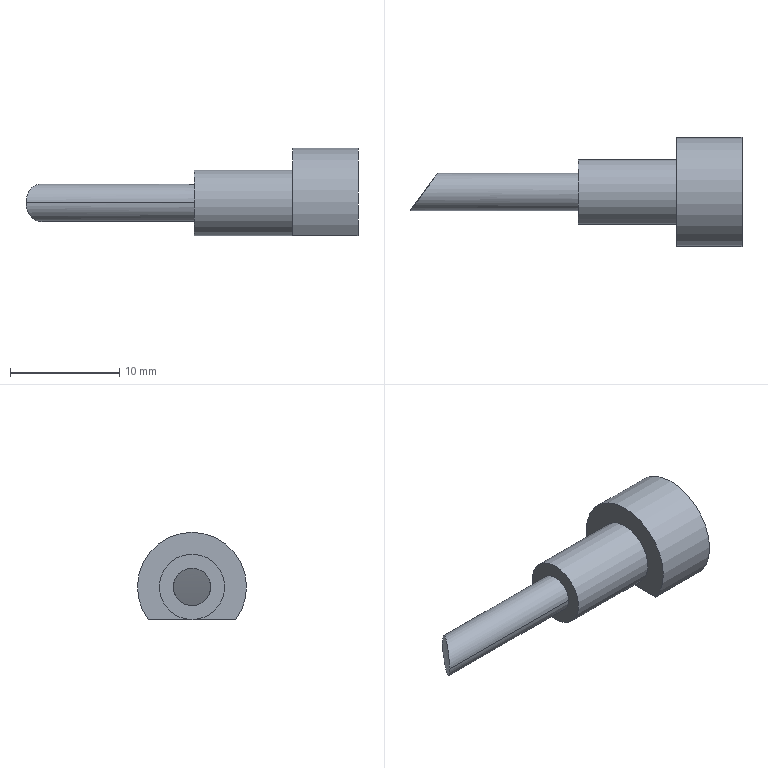Part | NX | features solid 2 | 1 solid | 9 faces | box 30.445 x 10 x 8 mm | volume 788.338 mm3 | cylinder 5 | plane 4 | commonest cylinder face diameters 3.417 x2 6 x1 10 x1 102.007 x1
STEP:
#1=CARTESIAN_POINT('',(64.275,-34.15,15.775));
#2=VERTEX_POINT('',#1);
#3=CARTESIAN_POINT('',(64.275,-26.15,15.775));
#4=VERTEX_POINT('',#3);
#5=CARTESIAN_POINT('',(64.275,-30.15,18.775));
#6=DIRECTION('',(-1.,0.,0.));
#7=DIRECTION('',(0.,0.,1.));
#8=AXIS2_PLACEMENT_3D('',#5,#6,#7);
#9=CIRCLE('',#8,5.);
#10=EDGE_CURVE('',#2,#4,#9,.T.);
#11=ORIENTED_EDGE('',*,*,#10,.F.);
#12=CARTESIAN_POINT('',(70.275,-34.15,15.775));
#13=VERTEX_POINT('',#12);
#14=CARTESIAN_POINT('',(70.275,-34.15,15.775));
#15=DIRECTION('',(-1.,0.,0.));
#16=VECTOR('',#15,1000.);
#17=LINE('',#14,#16);
#18=EDGE_CURVE('',#2,#13,#17,.F.);
#19=ORIENTED_EDGE('',*,*,#18,.T.);
#20=CARTESIAN_POINT('',(70.275,-26.15,15.775));
#21=VERTEX_POINT('',#20);
#22=CARTESIAN_POINT('',(70.275,-30.15,18.775));
#23=DIRECTION('',(-1.,0.,0.));
#24=DIRECTION('',(0.,0.,1.));
#25=AXIS2_PLACEMENT_3D('',#22,#23,#24);
#26=CIRCLE('',#25,5.);
#27=EDGE_CURVE('',#13,#21,#26,.T.);
#28=ORIENTED_EDGE('',*,*,#27,.T.);
#29=CARTESIAN_POINT('',(70.275,-26.15,15.775));
#30=DIRECTION('',(-1.,0.,0.));
#31=VECTOR('',#30,1000.);
#32=LINE('',#29,#31);
#33=EDGE_CURVE('',#21,#4,#32,.T.);
#34=ORIENTED_EDGE('',*,*,#33,.T.);
#35=EDGE_LOOP('',(#11,#19,#28,#34));
#36=FACE_BOUND('',#35,.T.);
#37=CARTESIAN_POINT('',(70.275,-30.15,18.775));
#38=DIRECTION('',(-1.,0.,0.));
#39=DIRECTION('',(0.,0.,1.));
#40=AXIS2_PLACEMENT_3D('',#37,#38,#39);
#41=CYLINDRICAL_SURFACE('',#40,5.);
#42=ADVANCED_FACE('',(#36),#41,.T.);
#43=CARTESIAN_POINT('',(64.275,-30.15,15.775));
#44=VERTEX_POINT('',#43);
#45=CARTESIAN_POINT('',(64.275,-30.15,18.775));
#46=DIRECTION('',(1.,0.,0.));
#47=DIRECTION('',(0.,0.,-1.));
#48=AXIS2_PLACEMENT_3D('',#45,#46,#47);
#49=CIRCLE('',#48,3.);
#50=EDGE_CURVE('',#44,#44,#49,.T.);
#51=ORIENTED_EDGE('',*,*,#50,.F.);
#52=EDGE_LOOP('',(#51));
#53=FACE_BOUND('',#52,.T.);
#54=CARTESIAN_POINT('',(55.275,-30.15,15.775));
#55=VERTEX_POINT('',#54);
#56=CARTESIAN_POINT('',(55.275,-30.15,18.775));
#57=DIRECTION('',(1.,0.,0.));
#58=DIRECTION('',(0.,0.,-1.));
#59=AXIS2_PLACEMENT_3D('',#56,#57,#58);
#60=CIRCLE('',#59,3.);
#61=EDGE_CURVE('',#55,#55,#60,.F.);
#62=ORIENTED_EDGE('',*,*,#61,.F.);
#63=EDGE_LOOP('',(#62));
#64=FACE_BOUND('',#63,.T.);
#65=CARTESIAN_POINT('',(-39.725,-30.15,18.775));
#66=DIRECTION('',(1.,0.,0.));
#67=DIRECTION('',(0.,0.,-1.));
#68=AXIS2_PLACEMENT_3D('',#65,#66,#67);
#69=CYLINDRICAL_SURFACE('',#68,3.);
#70=ADVANCED_FACE('',(#53,#64),#69,.T.);
#71=ORIENTED_EDGE('',*,*,#61,.T.);
#72=EDGE_LOOP('',(#71));
#73=FACE_BOUND('',#72,.T.);
#74=CARTESIAN_POINT('',(55.275,-28.442,18.775));
#75=VERTEX_POINT('',#74);
#76=CARTESIAN_POINT('',(55.275,-31.858,18.775));
#77=VERTEX_POINT('',#76);
#78=CARTESIAN_POINT('',(55.275,-30.15,18.775));
#79=DIRECTION('',(-1.,0.,0.));
#80=DIRECTION('',(0.,1.,0.));
#81=AXIS2_PLACEMENT_3D('',#78,#79,#80);
#82=CIRCLE('',#81,1.708);
#83=EDGE_CURVE('',#75,#77,#82,.T.);
#84=ORIENTED_EDGE('',*,*,#83,.F.);
#85=CARTESIAN_POINT('',(55.275,-30.15,18.775));
#86=DIRECTION('',(-1.,0.,0.));
#87=DIRECTION('',(0.,-1.,0.));
#88=AXIS2_PLACEMENT_3D('',#85,#86,#87);
#89=CIRCLE('',#88,1.708);
#90=EDGE_CURVE('',#77,#75,#89,.T.);
#91=ORIENTED_EDGE('',*,*,#90,.F.);
#92=EDGE_LOOP('',(#84,#91));
#93=FACE_BOUND('',#92,.T.);
#94=CARTESIAN_POINT('',(55.275,0.,-24.942));
#95=DIRECTION('',(1.,0.,0.));
#96=DIRECTION('',(0.,0.,-1.));
#97=AXIS2_PLACEMENT_3D('',#94,#95,#96);
#98=PLANE('',#97);
#99=ADVANCED_FACE('',(#73,#93),#98,.F.);
#100=CARTESIAN_POINT('',(42.337,-28.442,18.775));
#101=VERTEX_POINT('',#100);
#102=CARTESIAN_POINT('',(55.275,-28.442,18.775));
#103=DIRECTION('',(-1.,0.000000001,-0.00000002));
#104=VECTOR('',#103,1000.);
#105=LINE('',#102,#104);
#106=EDGE_CURVE('',#101,#75,#105,.F.);
#107=ORIENTED_EDGE('',*,*,#106,.F.);
#108=CARTESIAN_POINT('',(39.83,-31.858,18.775));
#109=VERTEX_POINT('',#108);
#110=CARTESIAN_POINT('',(39.83,-31.858,18.775));
#111=CARTESIAN_POINT('',(39.83,-31.858,19.283));
#112=CARTESIAN_POINT('',(40.216,-31.379,20.199));
#113=CARTESIAN_POINT('',(41.132,-30.174,20.621));
#114=CARTESIAN_POINT('',(42.012,-28.93,20.219));
#115=CARTESIAN_POINT('',(42.337,-28.441,19.284));
#116=CARTESIAN_POINT('',(42.337,-28.442,18.775));
#117=B_SPLINE_CURVE_WITH_KNOTS('',3,(#110,#111,#112,#113,#114,#115,#116),.UNSPECIFIED.,.F.,.F.,(4,1,1,1,4),(0.,0.0015,0.003,0.0045,0.006),.UNSPECIFIED.);
#118=EDGE_CURVE('',#101,#109,#117,.F.);
#119=ORIENTED_EDGE('',*,*,#118,.T.);
#120=CARTESIAN_POINT('',(55.275,-31.858,18.775));
#121=DIRECTION('',(-1.,-0.000000007,0.000000045));
#122=VECTOR('',#121,1000.);
#123=LINE('',#120,#122);
#124=EDGE_CURVE('',#77,#109,#123,.T.);
#125=ORIENTED_EDGE('',*,*,#124,.F.);
#126=ORIENTED_EDGE('',*,*,#90,.T.);
#127=EDGE_LOOP('',(#107,#119,#125,#126));
#128=FACE_BOUND('',#127,.T.);
#129=CARTESIAN_POINT('',(55.275,-30.15,18.775));
#130=DIRECTION('',(1.,0.,0.));
#131=DIRECTION('',(0.,-1.,0.));
#132=AXIS2_PLACEMENT_3D('',#129,#130,#131);
#133=CYLINDRICAL_SURFACE('',#132,1.708);
#134=ADVANCED_FACE('',(#128),#133,.T.);
#135=ORIENTED_EDGE('',*,*,#124,.T.);
#136=CARTESIAN_POINT('',(42.337,-28.442,18.775));
#137=CARTESIAN_POINT('',(42.337,-28.442,18.267));
#138=CARTESIAN_POINT('',(42.013,-28.928,17.331));
#139=CARTESIAN_POINT('',(41.127,-30.18,16.93));
#140=CARTESIAN_POINT('',(40.22,-31.374,17.348));
#141=CARTESIAN_POINT('',(39.83,-31.859,18.266));
#142=CARTESIAN_POINT('',(39.83,-31.858,18.775));
#143=B_SPLINE_CURVE_WITH_KNOTS('',3,(#136,#137,#138,#139,#140,#141,#142),.UNSPECIFIED.,.F.,.F.,(4,1,1,1,4),(0.,0.0015,0.003001,0.004501,0.006002),.UNSPECIFIED.);
#144=EDGE_CURVE('',#109,#101,#143,.F.);
#145=ORIENTED_EDGE('',*,*,#144,.T.);
#146=ORIENTED_EDGE('',*,*,#106,.T.);
#147=ORIENTED_EDGE('',*,*,#83,.T.);
#148=EDGE_LOOP('',(#135,#145,#146,#147));
#149=FACE_BOUND('',#148,.T.);
#150=CARTESIAN_POINT('',(55.275,-30.15,18.775));
#151=DIRECTION('',(1.,0.,0.));
#152=DIRECTION('',(0.,-1.,0.));
#153=AXIS2_PLACEMENT_3D('',#150,#151,#152);
#154=CYLINDRICAL_SURFACE('',#153,1.708);
#155=ADVANCED_FACE('',(#149),#154,.T.);
#156=ORIENTED_EDGE('',*,*,#118,.F.);
#157=ORIENTED_EDGE('',*,*,#144,.F.);
#158=EDGE_LOOP('',(#156,#157));
#159=FACE_BOUND('',#158,.T.);
#160=CARTESIAN_POINT('',(0.,0.,31.84));
#161=DIRECTION('',(0.,0.,1.));
#162=DIRECTION('',(0.,-1.,0.));
#163=AXIS2_PLACEMENT_3D('',#160,#161,#162);
#164=CYLINDRICAL_SURFACE('',#163,51.004);
#165=ADVANCED_FACE('',(#159),#164,.F.);
#166=CARTESIAN_POINT('',(64.275,-30.15,15.775));
#167=DIRECTION('',(0.,-1.,0.));
#168=VECTOR('',#167,1000.);
#169=LINE('',#166,#168);
#170=EDGE_CURVE('',#44,#4,#169,.F.);
#171=ORIENTED_EDGE('',*,*,#170,.F.);
#172=ORIENTED_EDGE('',*,*,#50,.T.);
#173=CARTESIAN_POINT('',(64.275,-30.15,15.775));
#174=DIRECTION('',(0.,-1.,0.));
#175=VECTOR('',#174,1000.);
#176=LINE('',#173,#175);
#177=EDGE_CURVE('',#2,#44,#176,.F.);
#178=ORIENTED_EDGE('',*,*,#177,.F.);
#179=ORIENTED_EDGE('',*,*,#10,.T.);
#180=EDGE_LOOP('',(#171,#172,#178,#179));
#181=FACE_BOUND('',#180,.T.);
#182=CARTESIAN_POINT('',(64.275,-30.15,18.775));
#183=DIRECTION('',(1.,0.,0.));
#184=DIRECTION('',(0.,0.,-1.));
#185=AXIS2_PLACEMENT_3D('',#182,#183,#184);
#186=PLANE('',#185);
#187=ADVANCED_FACE('',(#181),#186,.F.);
#188=ORIENTED_EDGE('',*,*,#27,.F.);
#189=CARTESIAN_POINT('',(70.275,-30.15,15.775));
#190=DIRECTION('',(0.,1.,0.));
#191=VECTOR('',#190,1000.);
#192=LINE('',#189,#191);
#193=EDGE_CURVE('',#13,#21,#192,.T.);
#194=ORIENTED_EDGE('',*,*,#193,.T.);
#195=EDGE_LOOP('',(#188,#194));
#196=FACE_BOUND('',#195,.T.);
#197=CARTESIAN_POINT('',(70.275,0.,3.449));
#198=DIRECTION('',(-1.,0.,0.));
#199=DIRECTION('',(0.,0.,1.));
#200=AXIS2_PLACEMENT_3D('',#197,#198,#199);
#201=PLANE('',#200);
#202=ADVANCED_FACE('',(#196),#201,.F.);
#203=ORIENTED_EDGE('',*,*,#177,.T.);
#204=ORIENTED_EDGE('',*,*,#170,.T.);
#205=ORIENTED_EDGE('',*,*,#33,.F.);
#206=ORIENTED_EDGE('',*,*,#193,.F.);
#207=ORIENTED_EDGE('',*,*,#18,.F.);
#208=EDGE_LOOP('',(#203,#204,#205,#206,#207));
#209=FACE_BOUND('',#208,.T.);
#210=CARTESIAN_POINT('',(67.275,-30.15,15.775));
#211=DIRECTION('',(0.,0.,-1.));
#212=DIRECTION('',(1.,0.,0.));
#213=AXIS2_PLACEMENT_3D('',#210,#211,#212);
#214=PLANE('',#213);
#215=ADVANCED_FACE('',(#209),#214,.T.);
#216=CLOSED_SHELL('',(#42,#70,#99,#134,#155,#165,#187,#202,#215));
#217=MANIFOLD_SOLID_BREP('',#216);
#218=(LENGTH_UNIT()NAMED_UNIT(*)SI_UNIT(.MILLI.,.METRE.));
#219=UNCERTAINTY_MEASURE_WITH_UNIT(LENGTH_MEASURE(0.0508),#218,'','');
#220=(NAMED_UNIT(*)PLANE_ANGLE_UNIT()SI_UNIT($,.RADIAN.));
#221=(NAMED_UNIT(*)SI_UNIT($,.STERADIAN.)SOLID_ANGLE_UNIT());
#222=(GEOMETRIC_REPRESENTATION_CONTEXT(3)GLOBAL_UNCERTAINTY_ASSIGNED_CONTEXT((#219))GLOBAL_UNIT_ASSIGNED_CONTEXT((#218,#220,#221))REPRESENTATION_CONTEXT('',''));
#223=ADVANCED_BREP_SHAPE_REPRESENTATION('',(#217),#222);